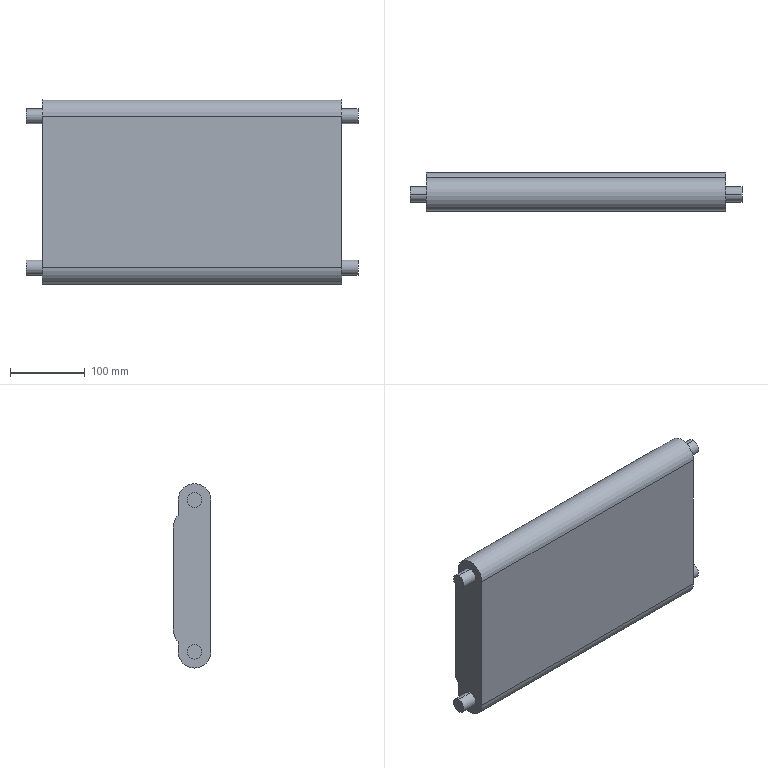Part | SolidWorks | features BaseBody 11, ICE 10, Chamfer 2 | 1 solid | 23 faces | box 444 x 50.745 x 246.557 mm | volume 4628488 mm3 | cylinder 13 | plane 10 | commonest cylinder face diameters 20 x8 44 x3 50 x2
STEP:
#1=CARTESIAN_POINT('',(38.124,30.841,937.301));
#2=VERTEX_POINT('',#1);
#3=CARTESIAN_POINT('',(38.124,30.841,917.301));
#4=VERTEX_POINT('',#3);
#5=CARTESIAN_POINT('',(38.124,30.841,927.301));
#6=DIRECTION('',(-1.,0.,0.));
#7=DIRECTION('',(0.,0.,1.));
#8=AXIS2_PLACEMENT_3D('',#5,#6,#7);
#9=CIRCLE('',#8,10.);
#10=EDGE_CURVE('',#2,#4,#9,.T.);
#11=ORIENTED_EDGE('',*,*,#10,.F.);
#12=CARTESIAN_POINT('',(60.124,30.841,937.301));
#13=VERTEX_POINT('',#12);
#14=CARTESIAN_POINT('',(38.124,30.841,937.301));
#15=DIRECTION('',(1.,0.,0.));
#16=VECTOR('',#15,1000.);
#17=LINE('',#14,#16);
#18=EDGE_CURVE('',#2,#13,#17,.T.);
#19=ORIENTED_EDGE('',*,*,#18,.T.);
#20=CARTESIAN_POINT('',(60.124,30.841,917.301));
#21=VERTEX_POINT('',#20);
#22=CARTESIAN_POINT('',(60.124,30.841,927.301));
#23=DIRECTION('',(-1.,0.,0.));
#24=DIRECTION('',(0.,0.,1.));
#25=AXIS2_PLACEMENT_3D('',#22,#23,#24);
#26=CIRCLE('',#25,10.);
#27=EDGE_CURVE('',#13,#21,#26,.T.);
#28=ORIENTED_EDGE('',*,*,#27,.T.);
#29=CARTESIAN_POINT('',(38.124,30.841,917.301));
#30=DIRECTION('',(1.,0.,0.));
#31=VECTOR('',#30,1000.);
#32=LINE('',#29,#31);
#33=EDGE_CURVE('',#4,#21,#32,.T.);
#34=ORIENTED_EDGE('',*,*,#33,.F.);
#35=EDGE_LOOP('',(#11,#19,#28,#34));
#36=FACE_OUTER_BOUND('',#35,.T.);
#37=CARTESIAN_POINT('',(38.124,30.841,927.301));
#38=DIRECTION('',(1.,0.,0.));
#39=DIRECTION('',(0.,0.,-1.));
#40=AXIS2_PLACEMENT_3D('',#37,#38,#39);
#41=CYLINDRICAL_SURFACE('',#40,10.);
#42=ADVANCED_FACE('',(#36),#41,.T.);
#43=CARTESIAN_POINT('',(38.124,30.841,734.744));
#44=VERTEX_POINT('',#43);
#45=CARTESIAN_POINT('',(38.124,30.841,714.744));
#46=VERTEX_POINT('',#45);
#47=CARTESIAN_POINT('',(38.124,30.841,724.744));
#48=DIRECTION('',(-1.,0.,0.));
#49=DIRECTION('',(0.,0.,1.));
#50=AXIS2_PLACEMENT_3D('',#47,#48,#49);
#51=CIRCLE('',#50,10.);
#52=EDGE_CURVE('',#44,#46,#51,.T.);
#53=ORIENTED_EDGE('',*,*,#52,.F.);
#54=CARTESIAN_POINT('',(60.124,30.841,734.744));
#55=VERTEX_POINT('',#54);
#56=CARTESIAN_POINT('',(38.124,30.841,734.744));
#57=DIRECTION('',(1.,0.,0.));
#58=VECTOR('',#57,1000.);
#59=LINE('',#56,#58);
#60=EDGE_CURVE('',#44,#55,#59,.T.);
#61=ORIENTED_EDGE('',*,*,#60,.T.);
#62=CARTESIAN_POINT('',(60.124,30.841,714.744));
#63=VERTEX_POINT('',#62);
#64=CARTESIAN_POINT('',(60.124,30.841,724.744));
#65=DIRECTION('',(-1.,0.,0.));
#66=DIRECTION('',(0.,0.,1.));
#67=AXIS2_PLACEMENT_3D('',#64,#65,#66);
#68=CIRCLE('',#67,10.);
#69=EDGE_CURVE('',#55,#63,#68,.T.);
#70=ORIENTED_EDGE('',*,*,#69,.T.);
#71=CARTESIAN_POINT('',(38.124,30.841,714.744));
#72=DIRECTION('',(1.,0.,0.));
#73=VECTOR('',#72,1000.);
#74=LINE('',#71,#73);
#75=EDGE_CURVE('',#46,#63,#74,.T.);
#76=ORIENTED_EDGE('',*,*,#75,.F.);
#77=EDGE_LOOP('',(#53,#61,#70,#76));
#78=FACE_OUTER_BOUND('',#77,.T.);
#79=CARTESIAN_POINT('',(38.124,30.841,724.744));
#80=DIRECTION('',(1.,0.,0.));
#81=DIRECTION('',(0.,0.,-1.));
#82=AXIS2_PLACEMENT_3D('',#79,#80,#81);
#83=CYLINDRICAL_SURFACE('',#82,10.);
#84=ADVANCED_FACE('',(#78),#83,.T.);
#85=CARTESIAN_POINT('',(482.124,30.841,917.301));
#86=VERTEX_POINT('',#85);
#87=CARTESIAN_POINT('',(482.124,30.841,937.301));
#88=VERTEX_POINT('',#87);
#89=CARTESIAN_POINT('',(482.124,30.841,927.301));
#90=DIRECTION('',(1.,0.,0.));
#91=DIRECTION('',(0.,0.,-1.));
#92=AXIS2_PLACEMENT_3D('',#89,#90,#91);
#93=CIRCLE('',#92,10.);
#94=EDGE_CURVE('',#86,#88,#93,.T.);
#95=ORIENTED_EDGE('',*,*,#94,.F.);
#96=CARTESIAN_POINT('',(460.124,30.841,917.301));
#97=VERTEX_POINT('',#96);
#98=CARTESIAN_POINT('',(482.124,30.841,917.301));
#99=DIRECTION('',(-1.,0.,0.));
#100=VECTOR('',#99,1000.);
#101=LINE('',#98,#100);
#102=EDGE_CURVE('',#86,#97,#101,.T.);
#103=ORIENTED_EDGE('',*,*,#102,.T.);
#104=CARTESIAN_POINT('',(460.124,30.841,937.301));
#105=VERTEX_POINT('',#104);
#106=CARTESIAN_POINT('',(460.124,30.841,927.301));
#107=DIRECTION('',(1.,0.,0.));
#108=DIRECTION('',(0.,0.,1.));
#109=AXIS2_PLACEMENT_3D('',#106,#107,#108);
#110=CIRCLE('',#109,10.);
#111=EDGE_CURVE('',#97,#105,#110,.T.);
#112=ORIENTED_EDGE('',*,*,#111,.T.);
#113=CARTESIAN_POINT('',(482.124,30.841,937.301));
#114=DIRECTION('',(-1.,0.,0.));
#115=VECTOR('',#114,1000.);
#116=LINE('',#113,#115);
#117=EDGE_CURVE('',#88,#105,#116,.T.);
#118=ORIENTED_EDGE('',*,*,#117,.F.);
#119=EDGE_LOOP('',(#95,#103,#112,#118));
#120=FACE_OUTER_BOUND('',#119,.T.);
#121=CARTESIAN_POINT('',(482.124,30.841,927.301));
#122=DIRECTION('',(-1.,0.,0.));
#123=DIRECTION('',(0.,0.,1.));
#124=AXIS2_PLACEMENT_3D('',#121,#122,#123);
#125=CYLINDRICAL_SURFACE('',#124,10.);
#126=ADVANCED_FACE('',(#120),#125,.T.);
#127=CARTESIAN_POINT('',(482.124,30.841,714.744));
#128=VERTEX_POINT('',#127);
#129=CARTESIAN_POINT('',(482.124,30.841,734.744));
#130=VERTEX_POINT('',#129);
#131=CARTESIAN_POINT('',(482.124,30.841,724.744));
#132=DIRECTION('',(1.,0.,0.));
#133=DIRECTION('',(0.,0.,-1.));
#134=AXIS2_PLACEMENT_3D('',#131,#132,#133);
#135=CIRCLE('',#134,10.);
#136=EDGE_CURVE('',#128,#130,#135,.T.);
#137=ORIENTED_EDGE('',*,*,#136,.F.);
#138=CARTESIAN_POINT('',(460.124,30.841,714.744));
#139=VERTEX_POINT('',#138);
#140=CARTESIAN_POINT('',(482.124,30.841,714.744));
#141=DIRECTION('',(-1.,0.,0.));
#142=VECTOR('',#141,1000.);
#143=LINE('',#140,#142);
#144=EDGE_CURVE('',#128,#139,#143,.T.);
#145=ORIENTED_EDGE('',*,*,#144,.T.);
#146=CARTESIAN_POINT('',(460.124,30.841,734.744));
#147=VERTEX_POINT('',#146);
#148=CARTESIAN_POINT('',(460.124,30.841,724.744));
#149=DIRECTION('',(1.,0.,0.));
#150=DIRECTION('',(0.,0.,1.));
#151=AXIS2_PLACEMENT_3D('',#148,#149,#150);
#152=CIRCLE('',#151,10.);
#153=EDGE_CURVE('',#139,#147,#152,.T.);
#154=ORIENTED_EDGE('',*,*,#153,.T.);
#155=CARTESIAN_POINT('',(482.124,30.841,734.744));
#156=DIRECTION('',(-1.,0.,0.));
#157=VECTOR('',#156,1000.);
#158=LINE('',#155,#157);
#159=EDGE_CURVE('',#130,#147,#158,.T.);
#160=ORIENTED_EDGE('',*,*,#159,.F.);
#161=EDGE_LOOP('',(#137,#145,#154,#160));
#162=FACE_OUTER_BOUND('',#161,.T.);
#163=CARTESIAN_POINT('',(482.124,30.841,724.744));
#164=DIRECTION('',(-1.,0.,0.));
#165=DIRECTION('',(0.,0.,1.));
#166=AXIS2_PLACEMENT_3D('',#163,#164,#165);
#167=CYLINDRICAL_SURFACE('',#166,10.);
#168=ADVANCED_FACE('',(#162),#167,.T.);
#169=CARTESIAN_POINT('',(60.124,30.841,702.744));
#170=VERTEX_POINT('',#169);
#171=CARTESIAN_POINT('',(60.124,8.841,724.744));
#172=VERTEX_POINT('',#171);
#173=CARTESIAN_POINT('',(60.124,30.841,724.744));
#174=DIRECTION('',(-1.,0.,0.));
#175=DIRECTION('',(0.,0.,-1.));
#176=AXIS2_PLACEMENT_3D('',#173,#174,#175);
#177=CIRCLE('',#176,22.);
#178=EDGE_CURVE('',#170,#172,#177,.T.);
#179=ORIENTED_EDGE('',*,*,#178,.F.);
#180=CARTESIAN_POINT('',(460.124,30.841,702.744));
#181=VERTEX_POINT('',#180);
#182=CARTESIAN_POINT('',(-190.328,30.841,702.744));
#183=DIRECTION('',(1.,0.,0.));
#184=VECTOR('',#183,1000.);
#185=LINE('',#182,#184);
#186=EDGE_CURVE('',#170,#181,#185,.T.);
#187=ORIENTED_EDGE('',*,*,#186,.T.);
#188=CARTESIAN_POINT('',(460.124,8.841,724.744));
#189=VERTEX_POINT('',#188);
#190=CARTESIAN_POINT('',(460.124,30.841,724.744));
#191=DIRECTION('',(-1.,0.,0.));
#192=DIRECTION('',(0.,0.,-1.));
#193=AXIS2_PLACEMENT_3D('',#190,#191,#192);
#194=CIRCLE('',#193,22.);
#195=EDGE_CURVE('',#181,#189,#194,.T.);
#196=ORIENTED_EDGE('',*,*,#195,.T.);
#197=CARTESIAN_POINT('',(-190.328,8.841,724.744));
#198=DIRECTION('',(-1.,0.,0.));
#199=VECTOR('',#198,1000.);
#200=LINE('',#197,#199);
#201=EDGE_CURVE('',#189,#172,#200,.T.);
#202=ORIENTED_EDGE('',*,*,#201,.T.);
#203=EDGE_LOOP('',(#179,#187,#196,#202));
#204=FACE_OUTER_BOUND('',#203,.T.);
#205=CARTESIAN_POINT('',(-190.328,30.841,724.744));
#206=DIRECTION('',(1.,0.,0.));
#207=DIRECTION('',(0.,0.,-1.));
#208=AXIS2_PLACEMENT_3D('',#205,#206,#207);
#209=CYLINDRICAL_SURFACE('',#208,22.);
#210=ADVANCED_FACE('',(#204),#209,.T.);
#211=ORIENTED_EDGE('',*,*,#201,.F.);
#212=CARTESIAN_POINT('',(460.124,8.841,927.301));
#213=VERTEX_POINT('',#212);
#214=CARTESIAN_POINT('',(460.124,8.841,724.744));
#215=DIRECTION('',(0.,0.,-1.));
#216=VECTOR('',#215,1000.);
#217=LINE('',#214,#216);
#218=EDGE_CURVE('',#213,#189,#217,.T.);
#219=ORIENTED_EDGE('',*,*,#218,.F.);
#220=CARTESIAN_POINT('',(60.124,8.841,927.301));
#221=VERTEX_POINT('',#220);
#222=CARTESIAN_POINT('',(-190.328,8.841,927.301));
#223=DIRECTION('',(1.,0.,0.));
#224=VECTOR('',#223,1000.);
#225=LINE('',#222,#224);
#226=EDGE_CURVE('',#221,#213,#225,.T.);
#227=ORIENTED_EDGE('',*,*,#226,.F.);
#228=CARTESIAN_POINT('',(60.124,8.841,724.744));
#229=DIRECTION('',(0.,0.,1.));
#230=VECTOR('',#229,1000.);
#231=LINE('',#228,#230);
#232=EDGE_CURVE('',#172,#221,#231,.T.);
#233=ORIENTED_EDGE('',*,*,#232,.F.);
#234=EDGE_LOOP('',(#211,#219,#227,#233));
#235=FACE_OUTER_BOUND('',#234,.T.);
#236=CARTESIAN_POINT('',(-190.328,8.841,724.744));
#237=DIRECTION('',(0.,1.,0.));
#238=DIRECTION('',(0.,0.,1.));
#239=AXIS2_PLACEMENT_3D('',#236,#237,#238);
#240=PLANE('',#239);
#241=ADVANCED_FACE('',(#235),#240,.F.);
#242=CARTESIAN_POINT('',(60.124,30.841,927.301));
#243=DIRECTION('',(-1.,0.,0.));
#244=DIRECTION('',(0.,0.,1.));
#245=AXIS2_PLACEMENT_3D('',#242,#243,#244);
#246=CIRCLE('',#245,10.);
#247=EDGE_CURVE('',#21,#13,#246,.T.);
#248=ORIENTED_EDGE('',*,*,#247,.F.);
#249=ORIENTED_EDGE('',*,*,#27,.F.);
#250=EDGE_LOOP('',(#248,#249));
#251=FACE_BOUND('',#250,.T.);
#252=CARTESIAN_POINT('',(60.124,30.841,724.744));
#253=DIRECTION('',(-1.,0.,0.));
#254=DIRECTION('',(0.,0.,1.));
#255=AXIS2_PLACEMENT_3D('',#252,#253,#254);
#256=CIRCLE('',#255,10.);
#257=EDGE_CURVE('',#63,#55,#256,.T.);
#258=ORIENTED_EDGE('',*,*,#257,.F.);
#259=ORIENTED_EDGE('',*,*,#69,.F.);
#260=EDGE_LOOP('',(#258,#259));
#261=FACE_BOUND('',#260,.T.);
#262=ORIENTED_EDGE('',*,*,#232,.T.);
#263=CARTESIAN_POINT('',(60.124,52.841,927.301));
#264=VERTEX_POINT('',#263);
#265=CARTESIAN_POINT('',(60.124,30.841,927.301));
#266=DIRECTION('',(-1.,0.,0.));
#267=DIRECTION('',(0.,0.,-1.));
#268=AXIS2_PLACEMENT_3D('',#265,#266,#267);
#269=CIRCLE('',#268,22.);
#270=EDGE_CURVE('',#221,#264,#269,.T.);
#271=ORIENTED_EDGE('',*,*,#270,.T.);
#272=CARTESIAN_POINT('',(60.124,52.841,907.188));
#273=VERTEX_POINT('',#272);
#274=CARTESIAN_POINT('',(60.124,52.841,724.744));
#275=DIRECTION('',(0.,0.,-1.));
#276=VECTOR('',#275,1000.);
#277=LINE('',#274,#276);
#278=EDGE_CURVE('',#264,#273,#277,.T.);
#279=ORIENTED_EDGE('',*,*,#278,.T.);
#280=CARTESIAN_POINT('',(60.124,59.585,890.108));
#281=VERTEX_POINT('',#280);
#282=CARTESIAN_POINT('',(60.124,34.585,890.108));
#283=DIRECTION('',(-1.,0.,0.));
#284=DIRECTION('',(0.,0.,-1.));
#285=AXIS2_PLACEMENT_3D('',#282,#283,#284);
#286=CIRCLE('',#285,25.);
#287=EDGE_CURVE('',#273,#281,#286,.T.);
#288=ORIENTED_EDGE('',*,*,#287,.T.);
#289=CARTESIAN_POINT('',(60.124,59.585,755.07));
#290=VERTEX_POINT('',#289);
#291=CARTESIAN_POINT('',(60.124,59.585,724.744));
#292=DIRECTION('',(0.,0.,-1.));
#293=VECTOR('',#292,1000.);
#294=LINE('',#291,#293);
#295=EDGE_CURVE('',#281,#290,#294,.T.);
#296=ORIENTED_EDGE('',*,*,#295,.T.);
#297=CARTESIAN_POINT('',(60.124,52.841,737.989));
#298=VERTEX_POINT('',#297);
#299=CARTESIAN_POINT('',(60.124,34.585,755.07));
#300=DIRECTION('',(-1.,0.,0.));
#301=DIRECTION('',(0.,0.,-1.));
#302=AXIS2_PLACEMENT_3D('',#299,#300,#301);
#303=CIRCLE('',#302,25.);
#304=EDGE_CURVE('',#290,#298,#303,.T.);
#305=ORIENTED_EDGE('',*,*,#304,.T.);
#306=CARTESIAN_POINT('',(60.124,52.841,724.744));
#307=VERTEX_POINT('',#306);
#308=CARTESIAN_POINT('',(60.124,52.841,724.744));
#309=DIRECTION('',(0.,0.,-1.));
#310=VECTOR('',#309,1000.);
#311=LINE('',#308,#310);
#312=EDGE_CURVE('',#298,#307,#311,.T.);
#313=ORIENTED_EDGE('',*,*,#312,.T.);
#314=CARTESIAN_POINT('',(60.124,30.841,724.744));
#315=DIRECTION('',(-1.,0.,0.));
#316=DIRECTION('',(0.,0.,-1.));
#317=AXIS2_PLACEMENT_3D('',#314,#315,#316);
#318=CIRCLE('',#317,22.);
#319=EDGE_CURVE('',#307,#170,#318,.T.);
#320=ORIENTED_EDGE('',*,*,#319,.T.);
#321=ORIENTED_EDGE('',*,*,#178,.T.);
#322=EDGE_LOOP('',(#262,#271,#279,#288,#296,#305,#313,#320,#321));
#323=FACE_OUTER_BOUND('',#322,.T.);
#324=CARTESIAN_POINT('',(60.124,30.841,724.744));
#325=DIRECTION('',(-1.,0.,0.));
#326=DIRECTION('',(0.,0.,1.));
#327=AXIS2_PLACEMENT_3D('',#324,#325,#326);
#328=PLANE('',#327);
#329=ADVANCED_FACE('',(#251,#261,#323),#328,.T.);
#330=ORIENTED_EDGE('',*,*,#186,.F.);
#331=ORIENTED_EDGE('',*,*,#319,.F.);
#332=CARTESIAN_POINT('',(460.124,52.841,724.744));
#333=VERTEX_POINT('',#332);
#334=CARTESIAN_POINT('',(-190.328,52.841,724.744));
#335=DIRECTION('',(1.,0.,0.));
#336=VECTOR('',#335,1000.);
#337=LINE('',#334,#336);
#338=EDGE_CURVE('',#307,#333,#337,.T.);
#339=ORIENTED_EDGE('',*,*,#338,.T.);
#340=CARTESIAN_POINT('',(460.124,30.841,724.744));
#341=DIRECTION('',(-1.,0.,0.));
#342=DIRECTION('',(0.,0.,-1.));
#343=AXIS2_PLACEMENT_3D('',#340,#341,#342);
#344=CIRCLE('',#343,22.);
#345=EDGE_CURVE('',#333,#181,#344,.T.);
#346=ORIENTED_EDGE('',*,*,#345,.T.);
#347=EDGE_LOOP('',(#330,#331,#339,#346));
#348=FACE_OUTER_BOUND('',#347,.T.);
#349=CARTESIAN_POINT('',(-190.328,30.841,724.744));
#350=DIRECTION('',(1.,0.,0.));
#351=DIRECTION('',(0.,0.,-1.));
#352=AXIS2_PLACEMENT_3D('',#349,#350,#351);
#353=CYLINDRICAL_SURFACE('',#352,22.);
#354=ADVANCED_FACE('',(#348),#353,.T.);
#355=CARTESIAN_POINT('',(460.124,30.841,927.301));
#356=DIRECTION('',(1.,0.,0.));
#357=DIRECTION('',(0.,0.,1.));
#358=AXIS2_PLACEMENT_3D('',#355,#356,#357);
#359=CIRCLE('',#358,10.);
#360=EDGE_CURVE('',#105,#97,#359,.T.);
#361=ORIENTED_EDGE('',*,*,#360,.F.);
#362=ORIENTED_EDGE('',*,*,#111,.F.);
#363=EDGE_LOOP('',(#361,#362));
#364=FACE_BOUND('',#363,.T.);
#365=CARTESIAN_POINT('',(460.124,30.841,724.744));
#366=DIRECTION('',(1.,0.,0.));
#367=DIRECTION('',(0.,0.,1.));
#368=AXIS2_PLACEMENT_3D('',#365,#366,#367);
#369=CIRCLE('',#368,10.);
#370=EDGE_CURVE('',#147,#139,#369,.T.);
#371=ORIENTED_EDGE('',*,*,#370,.F.);
#372=ORIENTED_EDGE('',*,*,#153,.F.);
#373=EDGE_LOOP('',(#371,#372));
#374=FACE_BOUND('',#373,.T.);
#375=CARTESIAN_POINT('',(460.124,59.585,755.07));
#376=VERTEX_POINT('',#375);
#377=CARTESIAN_POINT('',(460.124,52.841,737.989));
#378=VERTEX_POINT('',#377);
#379=CARTESIAN_POINT('',(460.124,34.585,755.07));
#380=DIRECTION('',(-1.,0.,0.));
#381=DIRECTION('',(0.,0.,-1.));
#382=AXIS2_PLACEMENT_3D('',#379,#380,#381);
#383=CIRCLE('',#382,25.);
#384=EDGE_CURVE('',#376,#378,#383,.T.);
#385=ORIENTED_EDGE('',*,*,#384,.F.);
#386=CARTESIAN_POINT('',(460.124,59.585,890.108));
#387=VERTEX_POINT('',#386);
#388=CARTESIAN_POINT('',(460.124,59.585,724.744));
#389=DIRECTION('',(0.,0.,-1.));
#390=VECTOR('',#389,1000.);
#391=LINE('',#388,#390);
#392=EDGE_CURVE('',#387,#376,#391,.T.);
#393=ORIENTED_EDGE('',*,*,#392,.F.);
#394=CARTESIAN_POINT('',(460.124,52.841,907.188));
#395=VERTEX_POINT('',#394);
#396=CARTESIAN_POINT('',(460.124,34.585,890.108));
#397=DIRECTION('',(-1.,0.,0.));
#398=DIRECTION('',(0.,0.,-1.));
#399=AXIS2_PLACEMENT_3D('',#396,#397,#398);
#400=CIRCLE('',#399,25.);
#401=EDGE_CURVE('',#395,#387,#400,.T.);
#402=ORIENTED_EDGE('',*,*,#401,.F.);
#403=CARTESIAN_POINT('',(460.124,52.841,927.301));
#404=VERTEX_POINT('',#403);
#405=CARTESIAN_POINT('',(460.124,52.841,724.744));
#406=DIRECTION('',(0.,0.,-1.));
#407=VECTOR('',#406,1000.);
#408=LINE('',#405,#407);
#409=EDGE_CURVE('',#404,#395,#408,.T.);
#410=ORIENTED_EDGE('',*,*,#409,.F.);
#411=CARTESIAN_POINT('',(460.124,30.841,927.301));
#412=DIRECTION('',(-1.,0.,0.));
#413=DIRECTION('',(0.,0.,-1.));
#414=AXIS2_PLACEMENT_3D('',#411,#412,#413);
#415=CIRCLE('',#414,22.);
#416=EDGE_CURVE('',#213,#404,#415,.T.);
#417=ORIENTED_EDGE('',*,*,#416,.F.);
#418=ORIENTED_EDGE('',*,*,#218,.T.);
#419=ORIENTED_EDGE('',*,*,#195,.F.);
#420=ORIENTED_EDGE('',*,*,#345,.F.);
#421=CARTESIAN_POINT('',(460.124,52.841,724.744));
#422=DIRECTION('',(0.,0.,-1.));
#423=VECTOR('',#422,1000.);
#424=LINE('',#421,#423);
#425=EDGE_CURVE('',#378,#333,#424,.T.);
#426=ORIENTED_EDGE('',*,*,#425,.F.);
#427=EDGE_LOOP('',(#385,#393,#402,#410,#417,#418,#419,#420,#426));
#428=FACE_OUTER_BOUND('',#427,.T.);
#429=CARTESIAN_POINT('',(460.124,30.841,724.744));
#430=DIRECTION('',(-1.,0.,0.));
#431=DIRECTION('',(0.,0.,1.));
#432=AXIS2_PLACEMENT_3D('',#429,#430,#431);
#433=PLANE('',#432);
#434=ADVANCED_FACE('',(#364,#374,#428),#433,.F.);
#435=ORIENTED_EDGE('',*,*,#416,.T.);
#436=CARTESIAN_POINT('',(-190.328,52.841,927.301));
#437=DIRECTION('',(-1.,0.,0.));
#438=VECTOR('',#437,1000.);
#439=LINE('',#436,#438);
#440=EDGE_CURVE('',#404,#264,#439,.T.);
#441=ORIENTED_EDGE('',*,*,#440,.T.);
#442=ORIENTED_EDGE('',*,*,#270,.F.);
#443=ORIENTED_EDGE('',*,*,#226,.T.);
#444=EDGE_LOOP('',(#435,#441,#442,#443));
#445=FACE_OUTER_BOUND('',#444,.T.);
#446=CARTESIAN_POINT('',(-190.328,30.841,927.301));
#447=DIRECTION('',(1.,0.,0.));
#448=DIRECTION('',(0.,0.,-1.));
#449=AXIS2_PLACEMENT_3D('',#446,#447,#448);
#450=CYLINDRICAL_SURFACE('',#449,22.);
#451=ADVANCED_FACE('',(#445),#450,.T.);
#452=CARTESIAN_POINT('',(-190.328,52.841,737.989));
#453=DIRECTION('',(-1.,0.,0.));
#454=VECTOR('',#453,1000.);
#455=LINE('',#452,#454);
#456=EDGE_CURVE('',#378,#298,#455,.T.);
#457=ORIENTED_EDGE('',*,*,#456,.F.);
#458=ORIENTED_EDGE('',*,*,#425,.T.);
#459=ORIENTED_EDGE('',*,*,#338,.F.);
#460=ORIENTED_EDGE('',*,*,#312,.F.);
#461=EDGE_LOOP('',(#457,#458,#459,#460));
#462=FACE_OUTER_BOUND('',#461,.T.);
#463=CARTESIAN_POINT('',(-190.328,52.841,724.744));
#464=DIRECTION('',(0.,-1.,0.));
#465=DIRECTION('',(0.,0.,-1.));
#466=AXIS2_PLACEMENT_3D('',#463,#464,#465);
#467=PLANE('',#466);
#468=ADVANCED_FACE('',(#462),#467,.F.);
#469=CARTESIAN_POINT('',(90.124,59.585,755.07));
#470=DIRECTION('',(1.,0.,0.));
#471=VECTOR('',#470,1000.);
#472=LINE('',#469,#471);
#473=EDGE_CURVE('',#290,#376,#472,.T.);
#474=ORIENTED_EDGE('',*,*,#473,.T.);
#475=ORIENTED_EDGE('',*,*,#384,.T.);
#476=ORIENTED_EDGE('',*,*,#456,.T.);
#477=ORIENTED_EDGE('',*,*,#304,.F.);
#478=EDGE_LOOP('',(#474,#475,#476,#477));
#479=FACE_OUTER_BOUND('',#478,.T.);
#480=CARTESIAN_POINT('',(90.124,34.585,755.07));
#481=DIRECTION('',(1.,0.,0.));
#482=DIRECTION('',(0.,0.,-1.));
#483=AXIS2_PLACEMENT_3D('',#480,#481,#482);
#484=CYLINDRICAL_SURFACE('',#483,25.);
#485=ADVANCED_FACE('',(#479),#484,.T.);
#486=ORIENTED_EDGE('',*,*,#392,.T.);
#487=ORIENTED_EDGE('',*,*,#473,.F.);
#488=ORIENTED_EDGE('',*,*,#295,.F.);
#489=CARTESIAN_POINT('',(90.124,59.585,890.108));
#490=DIRECTION('',(-1.,0.,0.));
#491=VECTOR('',#490,1000.);
#492=LINE('',#489,#491);
#493=EDGE_CURVE('',#387,#281,#492,.T.);
#494=ORIENTED_EDGE('',*,*,#493,.F.);
#495=EDGE_LOOP('',(#486,#487,#488,#494));
#496=FACE_OUTER_BOUND('',#495,.T.);
#497=CARTESIAN_POINT('',(90.124,59.585,890.108));
#498=DIRECTION('',(0.,-1.,0.));
#499=DIRECTION('',(0.,0.,-1.));
#500=AXIS2_PLACEMENT_3D('',#497,#498,#499);
#501=PLANE('',#500);
#502=ADVANCED_FACE('',(#496),#501,.F.);
#503=ORIENTED_EDGE('',*,*,#401,.T.);
#504=ORIENTED_EDGE('',*,*,#493,.T.);
#505=ORIENTED_EDGE('',*,*,#287,.F.);
#506=CARTESIAN_POINT('',(90.124,52.841,907.188));
#507=DIRECTION('',(1.,0.,0.));
#508=VECTOR('',#507,1000.);
#509=LINE('',#506,#508);
#510=EDGE_CURVE('',#273,#395,#509,.T.);
#511=ORIENTED_EDGE('',*,*,#510,.T.);
#512=EDGE_LOOP('',(#503,#504,#505,#511));
#513=FACE_OUTER_BOUND('',#512,.T.);
#514=CARTESIAN_POINT('',(90.124,34.585,890.108));
#515=DIRECTION('',(1.,0.,0.));
#516=DIRECTION('',(0.,0.,-1.));
#517=AXIS2_PLACEMENT_3D('',#514,#515,#516);
#518=CYLINDRICAL_SURFACE('',#517,25.);
#519=ADVANCED_FACE('',(#513),#518,.T.);
#520=ORIENTED_EDGE('',*,*,#278,.F.);
#521=ORIENTED_EDGE('',*,*,#440,.F.);
#522=ORIENTED_EDGE('',*,*,#409,.T.);
#523=ORIENTED_EDGE('',*,*,#510,.F.);
#524=EDGE_LOOP('',(#520,#521,#522,#523));
#525=FACE_OUTER_BOUND('',#524,.T.);
#526=CARTESIAN_POINT('',(-190.328,52.841,724.744));
#527=DIRECTION('',(0.,-1.,0.));
#528=DIRECTION('',(0.,0.,-1.));
#529=AXIS2_PLACEMENT_3D('',#526,#527,#528);
#530=PLANE('',#529);
#531=ADVANCED_FACE('',(#525),#530,.F.);
#532=ORIENTED_EDGE('',*,*,#144,.F.);
#533=CARTESIAN_POINT('',(482.124,30.841,724.744));
#534=DIRECTION('',(1.,0.,0.));
#535=DIRECTION('',(0.,0.,-1.));
#536=AXIS2_PLACEMENT_3D('',#533,#534,#535);
#537=CIRCLE('',#536,10.);
#538=EDGE_CURVE('',#130,#128,#537,.T.);
#539=ORIENTED_EDGE('',*,*,#538,.F.);
#540=ORIENTED_EDGE('',*,*,#159,.T.);
#541=ORIENTED_EDGE('',*,*,#370,.T.);
#542=EDGE_LOOP('',(#532,#539,#540,#541));
#543=FACE_OUTER_BOUND('',#542,.T.);
#544=CARTESIAN_POINT('',(482.124,30.841,724.744));
#545=DIRECTION('',(-1.,0.,0.));
#546=DIRECTION('',(0.,0.,1.));
#547=AXIS2_PLACEMENT_3D('',#544,#545,#546);
#548=CYLINDRICAL_SURFACE('',#547,10.);
#549=ADVANCED_FACE('',(#543),#548,.T.);
#550=ORIENTED_EDGE('',*,*,#538,.T.);
#551=ORIENTED_EDGE('',*,*,#136,.T.);
#552=EDGE_LOOP('',(#550,#551));
#553=FACE_OUTER_BOUND('',#552,.T.);
#554=CARTESIAN_POINT('',(482.124,30.841,724.744));
#555=DIRECTION('',(1.,0.,0.));
#556=DIRECTION('',(0.,0.,-1.));
#557=AXIS2_PLACEMENT_3D('',#554,#555,#556);
#558=PLANE('',#557);
#559=ADVANCED_FACE('',(#553),#558,.T.);
#560=ORIENTED_EDGE('',*,*,#102,.F.);
#561=CARTESIAN_POINT('',(482.124,30.841,927.301));
#562=DIRECTION('',(1.,0.,0.));
#563=DIRECTION('',(0.,0.,-1.));
#564=AXIS2_PLACEMENT_3D('',#561,#562,#563);
#565=CIRCLE('',#564,10.);
#566=EDGE_CURVE('',#88,#86,#565,.T.);
#567=ORIENTED_EDGE('',*,*,#566,.F.);
#568=ORIENTED_EDGE('',*,*,#117,.T.);
#569=ORIENTED_EDGE('',*,*,#360,.T.);
#570=EDGE_LOOP('',(#560,#567,#568,#569));
#571=FACE_OUTER_BOUND('',#570,.T.);
#572=CARTESIAN_POINT('',(482.124,30.841,927.301));
#573=DIRECTION('',(-1.,0.,0.));
#574=DIRECTION('',(0.,0.,1.));
#575=AXIS2_PLACEMENT_3D('',#572,#573,#574);
#576=CYLINDRICAL_SURFACE('',#575,10.);
#577=ADVANCED_FACE('',(#571),#576,.T.);
#578=ORIENTED_EDGE('',*,*,#566,.T.);
#579=ORIENTED_EDGE('',*,*,#94,.T.);
#580=EDGE_LOOP('',(#578,#579));
#581=FACE_OUTER_BOUND('',#580,.T.);
#582=CARTESIAN_POINT('',(482.124,30.841,927.301));
#583=DIRECTION('',(1.,0.,0.));
#584=DIRECTION('',(0.,0.,-1.));
#585=AXIS2_PLACEMENT_3D('',#582,#583,#584);
#586=PLANE('',#585);
#587=ADVANCED_FACE('',(#581),#586,.T.);
#588=ORIENTED_EDGE('',*,*,#60,.F.);
#589=CARTESIAN_POINT('',(38.124,30.841,724.744));
#590=DIRECTION('',(-1.,0.,0.));
#591=DIRECTION('',(0.,0.,1.));
#592=AXIS2_PLACEMENT_3D('',#589,#590,#591);
#593=CIRCLE('',#592,10.);
#594=EDGE_CURVE('',#46,#44,#593,.T.);
#595=ORIENTED_EDGE('',*,*,#594,.F.);
#596=ORIENTED_EDGE('',*,*,#75,.T.);
#597=ORIENTED_EDGE('',*,*,#257,.T.);
#598=EDGE_LOOP('',(#588,#595,#596,#597));
#599=FACE_OUTER_BOUND('',#598,.T.);
#600=CARTESIAN_POINT('',(38.124,30.841,724.744));
#601=DIRECTION('',(1.,0.,0.));
#602=DIRECTION('',(0.,0.,-1.));
#603=AXIS2_PLACEMENT_3D('',#600,#601,#602);
#604=CYLINDRICAL_SURFACE('',#603,10.);
#605=ADVANCED_FACE('',(#599),#604,.T.);
#606=ORIENTED_EDGE('',*,*,#594,.T.);
#607=ORIENTED_EDGE('',*,*,#52,.T.);
#608=EDGE_LOOP('',(#606,#607));
#609=FACE_OUTER_BOUND('',#608,.T.);
#610=CARTESIAN_POINT('',(38.124,30.841,724.744));
#611=DIRECTION('',(-1.,0.,0.));
#612=DIRECTION('',(0.,0.,1.));
#613=AXIS2_PLACEMENT_3D('',#610,#611,#612);
#614=PLANE('',#613);
#615=ADVANCED_FACE('',(#609),#614,.T.);
#616=ORIENTED_EDGE('',*,*,#18,.F.);
#617=CARTESIAN_POINT('',(38.124,30.841,927.301));
#618=DIRECTION('',(-1.,0.,0.));
#619=DIRECTION('',(0.,0.,1.));
#620=AXIS2_PLACEMENT_3D('',#617,#618,#619);
#621=CIRCLE('',#620,10.);
#622=EDGE_CURVE('',#4,#2,#621,.T.);
#623=ORIENTED_EDGE('',*,*,#622,.F.);
#624=ORIENTED_EDGE('',*,*,#33,.T.);
#625=ORIENTED_EDGE('',*,*,#247,.T.);
#626=EDGE_LOOP('',(#616,#623,#624,#625));
#627=FACE_OUTER_BOUND('',#626,.T.);
#628=CARTESIAN_POINT('',(38.124,30.841,927.301));
#629=DIRECTION('',(1.,0.,0.));
#630=DIRECTION('',(0.,0.,-1.));
#631=AXIS2_PLACEMENT_3D('',#628,#629,#630);
#632=CYLINDRICAL_SURFACE('',#631,10.);
#633=ADVANCED_FACE('',(#627),#632,.T.);
#634=ORIENTED_EDGE('',*,*,#622,.T.);
#635=ORIENTED_EDGE('',*,*,#10,.T.);
#636=EDGE_LOOP('',(#634,#635));
#637=FACE_OUTER_BOUND('',#636,.T.);
#638=CARTESIAN_POINT('',(38.124,30.841,927.301));
#639=DIRECTION('',(-1.,0.,0.));
#640=DIRECTION('',(0.,0.,1.));
#641=AXIS2_PLACEMENT_3D('',#638,#639,#640);
#642=PLANE('',#641);
#643=ADVANCED_FACE('',(#637),#642,.T.);
#644=CLOSED_SHELL('',(#42,#84,#126,#168,#210,#241,#329,#354,#434,#451,#468,#485,#502,#519,#531,#549,#559,#577,#587,#605,#615,#633,#643));
#645=MANIFOLD_SOLID_BREP('',#644);
#646=CARTESIAN_POINT('',(0.,0.,0.));
#647=DIRECTION('',(0.,0.,1.));
#648=DIRECTION('',(1.,0.,0.));
#649=AXIS2_PLACEMENT_3D('',#646,#647,#648);
#650=(LENGTH_UNIT()NAMED_UNIT(*)SI_UNIT(.MILLI.,.METRE.));
#651=UNCERTAINTY_MEASURE_WITH_UNIT(LENGTH_MEASURE(0.00001),#650,'','');
#652=(NAMED_UNIT(*)PLANE_ANGLE_UNIT()SI_UNIT($,.RADIAN.));
#653=(NAMED_UNIT(*)SI_UNIT($,.STERADIAN.)SOLID_ANGLE_UNIT());
#654=(GEOMETRIC_REPRESENTATION_CONTEXT(3)GLOBAL_UNCERTAINTY_ASSIGNED_CONTEXT((#651))GLOBAL_UNIT_ASSIGNED_CONTEXT((#650,#652,#653))REPRESENTATION_CONTEXT('',''));
#655=ADVANCED_BREP_SHAPE_REPRESENTATION('',(#645,#649),#654);